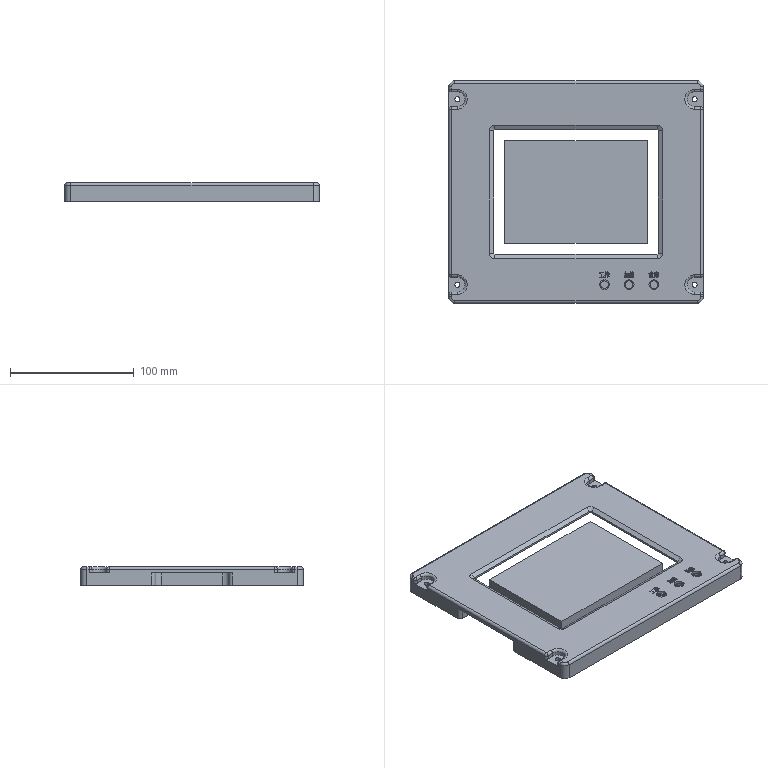NC program | Mastercam | posted with a generic post | part box 206 x 180 x 15 mm
Lines 737 to 1835 of 42274:
(4 BNOS |TOOL - 1|DIA. OFF. - 1|LEN. - 1|TOOL DIA. - 4.)
N1542 T1 M6
N1544 G0 G54 G90 X68.664 Y49.5 C0. B0. S10000 M3
N1546 G43 H1 Z24.953
N1548 Z4.953
N1550 G1 Z-.047 F600.
N1552 X68.643 Y49.851 F4000.
N1554 X68.576 Y50.211
N1556 X68.459 Y50.573
N1558 X68.339 Y50.838
N1560 X68.189 Y51.095
N1562 X68.012 Y51.337
N1564 X67.811 Y51.561
N1566 X67.587 Y51.762
N1568 X67.345 Y51.939
N1570 X67.088 Y52.089
N1572 X66.823 Y52.209
N1574 X66.461 Y52.326
N1576 X66.101 Y52.393
N1578 X65.75 Y52.414
N1580 X-65.75
N1582 X-66.101 Y52.393
N1584 X-66.461 Y52.326
N1586 X-66.823 Y52.209
N1588 X-67.088 Y52.089
N1590 X-67.345 Y51.939
N1592 X-67.587 Y51.762
N1594 X-67.811 Y51.561
N1596 X-68.012 Y51.337
N1598 X-68.189 Y51.095
N1600 X-68.339 Y50.838
N1602 X-68.459 Y50.573
N1604 X-68.576 Y50.211
N1606 X-68.643 Y49.851
N1608 X-68.664 Y49.5
N1610 Y-49.5
N1612 X-68.347
N1614 Z-.231
N1616 Y49.5
N1618 X-68.328 Y49.813
N1620 X-68.268 Y50.134
N1622 X-68.164 Y50.456
N1624 X-68.056 Y50.693
N1626 X-67.923 Y50.921
N1628 X-67.766 Y51.137
N1630 X-67.586 Y51.336
N1632 X-67.387 Y51.516
N1634 X-67.171 Y51.673
N1636 X-66.943 Y51.806
N1638 X-66.706 Y51.914
N1640 X-66.384 Y52.018
N1642 X-66.063 Y52.078
N1644 X-65.75 Y52.097
N1646 X65.75
N1648 X66.063 Y52.078
N1650 X66.384 Y52.018
N1652 X66.706 Y51.914
N1654 X66.943 Y51.806
N1656 X67.171 Y51.673
N1658 X67.387 Y51.516
N1660 X67.586 Y51.336
N1662 X67.766 Y51.137
N1664 X67.923 Y50.921
N1666 X68.056 Y50.693
N1668 X68.164 Y50.456
N1670 X68.268 Y50.134
N1672 X68.328 Y49.813
N1674 X68.347 Y49.5
N1676 Y-49.5
N1678 X68.328 Y-49.813
N1680 X68.268 Y-50.134
N1682 X68.164 Y-50.456
N1684 X68.056 Y-50.693
N1686 X67.923 Y-50.921
N1688 X67.766 Y-51.137
N1690 X67.586 Y-51.336
N1692 X67.387 Y-51.516
N1694 X67.171 Y-51.673
N1696 X66.943 Y-51.806
N1698 X66.706 Y-51.914
N1700 X66.384 Y-52.018
N1702 X66.063 Y-52.078
N1704 X65.75 Y-52.097
N1706 X-65.75
N1708 X-66.063 Y-52.078
N1710 X-66.384 Y-52.018
N1712 X-66.706 Y-51.914
N1714 X-66.943 Y-51.806
N1716 X-67.171 Y-51.673
N1718 X-67.387 Y-51.516
N1720 X-67.586 Y-51.336
N1722 X-67.766 Y-51.137
N1724 X-67.923 Y-50.921
N1726 X-68.056 Y-50.693
N1728 X-68.164 Y-50.456
N1730 X-68.268 Y-50.134
N1732 X-68.328 Y-49.813
N1734 X-68.347 Y-49.5
N1736 X-68.058
N1738 Z-.397
N1740 X-68.041 Y-49.778
N1742 X-67.988 Y-50.063
N1744 X-67.896 Y-50.35
N1746 X-67.8 Y-50.56
N1748 X-67.682 Y-50.763
N1750 X-67.542 Y-50.955
N1752 X-67.382 Y-51.132
N1754 X-67.205 Y-51.292
N1756 X-67.013 Y-51.432
N1758 X-66.81 Y-51.55
N1760 X-66.6 Y-51.646
N1762 X-66.313 Y-51.738
N1764 X-66.028 Y-51.791
N1766 X-65.75 Y-51.808
N1768 X65.75
N1770 X66.028 Y-51.791
N1772 X66.313 Y-51.738
N1774 X66.6 Y-51.646
N1776 X66.81 Y-51.55
N1778 X67.013 Y-51.432
N1780 X67.205 Y-51.292
N1782 X67.382 Y-51.132
N1784 X67.542 Y-50.955
N1786 X67.682 Y-50.763
N1788 X67.8 Y-50.56
N1790 X67.896 Y-50.35
N1792 X67.988 Y-50.063
N1794 X68.041 Y-49.778
N1796 X68.058 Y-49.5
N1798 Y49.5
N1800 X68.041 Y49.778
N1802 X67.988 Y50.063
N1804 X67.896 Y50.35
N1806 X67.8 Y50.56
N1808 X67.682 Y50.763
N1810 X67.542 Y50.955
N1812 X67.382 Y51.132
N1814 X67.205 Y51.292
N1816 X67.013 Y51.432
N1818 X66.81 Y51.55
N1820 X66.6 Y51.646
N1822 X66.313 Y51.738
N1824 X66.028 Y51.791
N1826 X65.75 Y51.808
N1828 X-65.75
N1830 X-66.028 Y51.791
N1832 X-66.313 Y51.738
N1834 X-66.6 Y51.646
N1836 X-66.81 Y51.55
N1838 X-67.013 Y51.432
N1840 X-67.205 Y51.292
N1842 X-67.382 Y51.132
N1844 X-67.542 Y50.955
N1846 X-67.682 Y50.763
N1848 X-67.8 Y50.56
N1850 X-67.896 Y50.35
N1852 X-67.988 Y50.063
N1854 X-68.041 Y49.778
N1856 X-68.058 Y49.5
N1858 Y-49.5
N1860 X-67.74
N1862 Z-.581
N1864 Y49.5
N1866 X-67.726 Y49.74
N1868 X-67.68 Y49.986
N1870 X-67.601 Y50.233
N1872 X-67.518 Y50.414
N1874 X-67.416 Y50.589
N1876 X-67.295 Y50.755
N1878 X-67.157 Y50.907
N1880 X-67.005 Y51.045
N1882 X-66.839 Y51.166
N1884 X-66.664 Y51.268
N1886 X-66.483 Y51.351
N1888 X-66.236 Y51.43
N1890 X-65.99 Y51.476
N1892 X-65.75 Y51.49
N1894 X65.75
N1896 X65.99 Y51.476
N1898 X66.236 Y51.43
N1900 X66.483 Y51.351
N1902 X66.664 Y51.268
N1904 X66.839 Y51.166
N1906 X67.005 Y51.045
N1908 X67.157 Y50.907
N1910 X67.295 Y50.755
N1912 X67.416 Y50.589
N1914 X67.518 Y50.414
N1916 X67.601 Y50.233
N1918 X67.68 Y49.986
N1920 X67.726 Y49.74
N1922 X67.74 Y49.5
N1924 Y-49.5
N1926 X67.726 Y-49.74
N1928 X67.68 Y-49.986
N1930 X67.601 Y-50.233
N1932 X67.518 Y-50.414
N1934 X67.416 Y-50.589
N1936 X67.295 Y-50.755
N1938 X67.157 Y-50.907
N1940 X67.005 Y-51.045
N1942 X66.839 Y-51.166
N1944 X66.664 Y-51.268
N1946 X66.483 Y-51.351
N1948 X66.236 Y-51.43
N1950 X65.99 Y-51.476
N1952 X65.75 Y-51.49
N1954 X-65.75
N1956 X-65.99 Y-51.476
N1958 X-66.236 Y-51.43
N1960 X-66.483 Y-51.351
N1962 X-66.664 Y-51.268
N1964 X-66.839 Y-51.166
N1966 X-67.005 Y-51.045
N1968 X-67.157 Y-50.907
N1970 X-67.295 Y-50.755
N1972 X-67.416 Y-50.589
N1974 X-67.518 Y-50.414
N1976 X-67.601 Y-50.233
N1978 X-67.68 Y-49.986
N1980 X-67.726 Y-49.74
N1982 X-67.74 Y-49.5
N1984 X-67.423
N1986 Z-.764
N1988 X-67.411 Y-49.701
N1990 X-67.372 Y-49.908
N1992 X-67.305 Y-50.116
N1994 X-67.236 Y-50.268
N1996 X-67.15 Y-50.415
N1998 X-67.049 Y-50.554
N2000 X-66.933 Y-50.683
N2002 X-66.804 Y-50.799
N2004 X-66.665 Y-50.9
N2006 X-66.518 Y-50.986
N2008 X-66.366 Y-51.055
N2010 X-66.158 Y-51.122
N2012 X-65.951 Y-51.161
N2014 X-65.75 Y-51.173
N2016 X65.75
N2018 X65.951 Y-51.161
N2020 X66.158 Y-51.122
N2022 X66.366 Y-51.055
N2024 X66.518 Y-50.986
N2026 X66.665 Y-50.9
N2028 X66.804 Y-50.799
N2030 X66.933 Y-50.683
N2032 X67.049 Y-50.554
N2034 X67.15 Y-50.415
N2036 X67.236 Y-50.268
N2038 X67.305 Y-50.116
N2040 X67.372 Y-49.908
N2042 X67.411 Y-49.701
N2044 X67.423 Y-49.5
N2046 Y49.5
N2048 X67.411 Y49.701
N2050 X67.372 Y49.908
N2052 X67.305 Y50.116
N2054 X67.236 Y50.268
N2056 X67.15 Y50.415
N2058 X67.049 Y50.554
N2060 X66.933 Y50.683
N2062 X66.804 Y50.799
N2064 X66.665 Y50.9
N2066 X66.518 Y50.986
N2068 X66.366 Y51.055
N2070 X66.158 Y51.122
N2072 X65.951 Y51.161
N2074 X65.75 Y51.173
N2076 X-65.75
N2078 X-65.951 Y51.161
N2080 X-66.158 Y51.122
N2082 X-66.366 Y51.055
N2084 X-66.518 Y50.986
N2086 X-66.665 Y50.9
N2088 X-66.804 Y50.799
N2090 X-66.933 Y50.683
N2092 X-67.049 Y50.554
N2094 X-67.15 Y50.415
N2096 X-67.236 Y50.268
N2098 X-67.305 Y50.116
N2100 X-67.372 Y49.908
N2102 X-67.411 Y49.701
N2104 X-67.423 Y49.5
N2106 Y-49.5
N2108 X-67.105
N2110 Z-.947
N2112 Y49.5
N2114 X-67.095 Y49.663
N2116 X-67.064 Y49.831
N2118 X-67.01 Y49.999
N2120 X-66.954 Y50.122
N2122 X-66.884 Y50.242
N2124 X-66.802 Y50.354
N2126 X-66.708 Y50.458
N2128 X-66.604 Y50.552
N2130 X-66.492 Y50.634
N2132 X-66.372 Y50.704
N2134 X-66.249 Y50.76
N2136 X-66.081 Y50.814
N2138 X-65.913 Y50.845
N2140 X-65.75 Y50.855
N2142 X65.75
N2144 X65.913 Y50.845
N2146 X66.081 Y50.814
N2148 X66.249 Y50.76
N2150 X66.372 Y50.704
N2152 X66.492 Y50.634
N2154 X66.604 Y50.552
N2156 X66.708 Y50.458
N2158 X66.802 Y50.354
N2160 X66.884 Y50.242
N2162 X66.954 Y50.122
N2164 X67.01 Y49.999
N2166 X67.064 Y49.831
N2168 X67.095 Y49.663
N2170 X67.105 Y49.5
N2172 Y-49.5
N2174 X67.095 Y-49.663
N2176 X67.064 Y-49.831
N2178 X67.01 Y-49.999
N2180 X66.954 Y-50.122
N2182 X66.884 Y-50.242
N2184 X66.802 Y-50.354
N2186 X66.708 Y-50.458
N2188 X66.604 Y-50.552
N2190 X66.492 Y-50.634
N2192 X66.372 Y-50.704
N2194 X66.249 Y-50.76
N2196 X66.081 Y-50.814
N2198 X65.913 Y-50.845
N2200 X65.75 Y-50.855
N2202 X-65.75
N2204 X-65.913 Y-50.845
N2206 X-66.081 Y-50.814
N2208 X-66.249 Y-50.76
N2210 X-66.372 Y-50.704
N2212 X-66.492 Y-50.634
N2214 X-66.604 Y-50.552
N2216 X-66.708 Y-50.458
N2218 X-66.802 Y-50.354
N2220 X-66.884 Y-50.242
N2222 X-66.954 Y-50.122
N2224 X-67.01 Y-49.999
N2226 X-67.064 Y-49.831
N2228 X-67.095 Y-49.663
N2230 X-67.105 Y-49.5
N2232 X-66.788
N2234 Z-1.131
N2236 X-66.78 Y-49.625
N2238 X-66.756 Y-49.753
N2240 X-66.715 Y-49.882
N2242 X-66.672 Y-49.977
N2244 X-66.619 Y-50.068
N2246 X-66.556 Y-50.154
N2248 X-66.484 Y-50.234
N2250 X-66.404 Y-50.306
N2252 X-66.318 Y-50.369
N2254 X-66.227 Y-50.422
N2256 X-66.132 Y-50.465
N2258 X-66.003 Y-50.506
N2260 X-65.875 Y-50.53
N2262 X-65.75 Y-50.538
N2264 X65.75
N2266 X65.875 Y-50.53
N2268 X66.003 Y-50.506
N2270 X66.132 Y-50.465
N2272 X66.227 Y-50.422
N2274 X66.318 Y-50.369
N2276 X66.404 Y-50.306
N2278 X66.484 Y-50.234
N2280 X66.556 Y-50.154
N2282 X66.619 Y-50.068
N2284 X66.672 Y-49.977
N2286 X66.715 Y-49.882
N2288 X66.756 Y-49.753
N2290 X66.78 Y-49.625
N2292 X66.788 Y-49.5
N2294 Y49.5
N2296 X66.78 Y49.625
N2298 X66.756 Y49.753
N2300 X66.715 Y49.882
N2302 X66.672 Y49.977
N2304 X66.619 Y50.068
N2306 X66.556 Y50.154
N2308 X66.484 Y50.234
N2310 X66.404 Y50.306
N2312 X66.318 Y50.369
N2314 X66.227 Y50.422
N2316 X66.132 Y50.465
N2318 X66.003 Y50.506
N2320 X65.875 Y50.53
N2322 X65.75 Y50.538
N2324 X-65.75
N2326 X-65.875 Y50.53
N2328 X-66.003 Y50.506
N2330 X-66.132 Y50.465
N2332 X-66.227 Y50.422
N2334 X-66.318 Y50.369
N2336 X-66.404 Y50.306
N2338 X-66.484 Y50.234
N2340 X-66.556 Y50.154
N2342 X-66.619 Y50.068
N2344 X-66.672 Y49.977
N2346 X-66.715 Y49.882
N2348 X-66.756 Y49.753
N2350 X-66.78 Y49.625
N2352 X-66.788 Y49.5
N2354 Y-49.5
N2356 X-66.47
N2358 Z-1.314
N2360 Y49.5
N2362 X-66.465 Y49.587
N2364 X-66.448 Y49.676
N2366 X-66.42 Y49.765
N2368 X-66.39 Y49.831
N2370 X-66.353 Y49.894
N2372 X-66.309 Y49.954
N2374 X-66.259 Y50.009
N2376 X-66.204 Y50.059
N2378 X-66.144 Y50.103
N2380 X-66.081 Y50.14
N2382 X-66.015 Y50.17
N2384 X-65.926 Y50.198
N2386 X-65.837 Y50.215
N2388 X-65.75 Y50.22
N2390 X65.75
N2392 X65.837 Y50.215
N2394 X65.926 Y50.198
N2396 X66.015 Y50.17
N2398 X66.081 Y50.14
N2400 X66.144 Y50.103
N2402 X66.204 Y50.059
N2404 X66.259 Y50.009
N2406 X66.309 Y49.954
N2408 X66.353 Y49.894
N2410 X66.39 Y49.831
N2412 X66.42 Y49.765
N2414 X66.448 Y49.676
N2416 X66.465 Y49.587
N2418 X66.47 Y49.5
N2420 Y-49.5
N2422 X66.465 Y-49.587
N2424 X66.448 Y-49.676
N2426 X66.42 Y-49.765
N2428 X66.39 Y-49.831
N2430 X66.353 Y-49.894
N2432 X66.309 Y-49.954
N2434 X66.259 Y-50.009
N2436 X66.204 Y-50.059
N2438 X66.144 Y-50.103
N2440 X66.081 Y-50.14
N2442 X66.015 Y-50.17
N2444 X65.926 Y-50.198
N2446 X65.837 Y-50.215
N2448 X65.75 Y-50.22
N2450 X-65.75
N2452 X-65.837 Y-50.215
N2454 X-65.926 Y-50.198
N2456 X-66.015 Y-50.17
N2458 X-66.081 Y-50.14
N2460 X-66.144 Y-50.103
N2462 X-66.204 Y-50.059
N2464 X-66.259 Y-50.009
N2466 X-66.309 Y-49.954
N2468 X-66.353 Y-49.894
N2470 X-66.39 Y-49.831
N2472 X-66.42 Y-49.765
N2474 X-66.448 Y-49.676
N2476 X-66.465 Y-49.587
N2478 X-66.47 Y-49.5
N2480 X-66.153
N2482 Z-1.497
N2484 X-66.15 Y-49.548
N2486 X-66.14 Y-49.598
N2488 X-66.124 Y-49.648
N2490 X-66.108 Y-49.685
N2492 X-66.087 Y-49.72
N2494 X-66.063 Y-49.754
N2496 X-66.035 Y-49.785
N2498 X-66.004 Y-49.813
N2500 X-65.97 Y-49.837
N2502 X-65.935 Y-49.858
N2504 X-65.898 Y-49.874
N2506 X-65.848 Y-49.89
N2508 X-65.798 Y-49.9
N2510 X-65.75 Y-49.903
N2512 X65.75
N2514 X65.798 Y-49.9
N2516 X65.848 Y-49.89
N2518 X65.898 Y-49.874
N2520 X65.935 Y-49.858
N2522 X65.97 Y-49.837
N2524 X66.004 Y-49.813
N2526 X66.035 Y-49.785
N2528 X66.063 Y-49.754
N2530 X66.087 Y-49.72
N2532 X66.108 Y-49.685
N2534 X66.124 Y-49.648
N2536 X66.14 Y-49.598
N2538 X66.15 Y-49.548
N2540 X66.153 Y-49.5
N2542 Y49.5
N2544 X66.15 Y49.548
N2546 X66.14 Y49.598
N2548 X66.124 Y49.648
N2550 X66.108 Y49.685
N2552 X66.087 Y49.72
N2554 X66.063 Y49.754
N2556 X66.035 Y49.785
N2558 X66.004 Y49.813
N2560 X65.97 Y49.837
N2562 X65.935 Y49.858
N2564 X65.898 Y49.874
N2566 X65.848 Y49.89
N2568 X65.798 Y49.9
N2570 X65.75 Y49.903
N2572 X-65.75
N2574 X-65.798 Y49.9
N2576 X-65.848 Y49.89
N2578 X-65.898 Y49.874
N2580 X-65.935 Y49.858
N2582 X-65.97 Y49.837
N2584 X-66.004 Y49.813
N2586 X-66.035 Y49.785
N2588 X-66.063 Y49.754
N2590 X-66.087 Y49.72
N2592 X-66.108 Y49.685
N2594 X-66.124 Y49.648
N2596 X-66.14 Y49.598
N2598 X-66.15 Y49.548
N2600 X-66.153 Y49.5
N2602 Y-49.5
N2604 X-65.835
N2606 Z-1.681
N2608 Y49.5
N2610 X-65.834 Y49.51
N2612 X-65.833 Y49.521
N2614 X-65.829 Y49.531
N2616 X-65.826 Y49.539
N2618 X-65.821 Y49.547
N2620 X-65.816 Y49.554
N2622 X-65.81 Y49.56
N2624 X-65.804 Y49.566
N2626 X-65.797 Y49.571
N2628 X-65.789 Y49.576
N2630 X-65.781 Y49.579
N2632 X-65.771 Y49.583
N2634 X-65.76 Y49.584
N2636 X-65.75 Y49.585
N2638 X65.75
N2640 X65.76 Y49.584
N2642 X65.771 Y49.583
N2644 X65.781 Y49.579
N2646 X65.789 Y49.576
N2648 X65.797 Y49.571
N2650 X65.804 Y49.566
N2652 X65.81 Y49.56
N2654 X65.816 Y49.554
N2656 X65.821 Y49.547
N2658 X65.826 Y49.539
N2660 X65.829 Y49.531
N2662 X65.833 Y49.521
N2664 X65.834 Y49.51
N2666 X65.835 Y49.5
N2668 Y-49.5
N2670 X65.834 Y-49.51
N2672 X65.833 Y-49.521
N2674 X65.829 Y-49.531
N2676 X65.826 Y-49.539
N2678 X65.821 Y-49.547
N2680 X65.816 Y-49.554
N2682 X65.81 Y-49.56
N2684 X65.804 Y-49.566
N2686 X65.797 Y-49.571
N2688 X65.789 Y-49.576
N2690 X65.781 Y-49.579
N2692 X65.771 Y-49.583
N2694 X65.76 Y-49.584
N2696 X65.75 Y-49.585
N2698 X-65.75
N2700 X-65.76 Y-49.584
N2702 X-65.771 Y-49.583
N2704 X-65.781 Y-49.579
N2706 X-65.789 Y-49.576
N2708 X-65.797 Y-49.571
N2710 X-65.804 Y-49.566
N2712 X-65.81 Y-49.56
N2714 X-65.816 Y-49.554
N2716 X-65.821 Y-49.547
N2718 X-65.826 Y-49.539
N2720 X-65.829 Y-49.531
N2722 X-65.833 Y-49.521
N2724 X-65.834 Y-49.51
N2726 X-65.835 Y-49.5
N2728 X-65.558 Y-49.268
N2730 Z-1.864
N2732 X65.518
N2734 Y49.268
N2736 X-65.518
N2738 Y-49.308
N2740 Z-1.846
N2742 X-65.2 Y-48.99
N2744 Z-2.047
N2746 Y48.95
N2748 X65.2
N2750 Y-48.95
N2752 X-65.24
N2754 G0 Z2.953
N2756 Z22.953
N2758 Z24.953
N2760 X-65.75 Y-52.414
N2762 Z4.953
N2764 G1 Z-.047 F600.
N2766 X-66.101 Y-52.393 F4000.
N2768 X-66.461 Y-52.326
N2770 X-66.823 Y-52.209
N2772 X-67.088 Y-52.089
N2774 X-67.345 Y-51.939
N2776 X-67.587 Y-51.762
N2778 X-67.811 Y-51.561
N2780 X-68.012 Y-51.337
N2782 X-68.189 Y-51.095
N2784 X-68.339 Y-50.838
N2786 X-68.459 Y-50.573
N2788 X-68.576 Y-50.211
N2790 X-68.643 Y-49.851
N2792 X-68.664 Y-49.5
N2794 G0 Z4.953
N2796 Z24.953
N2798 X-65.75 Y-52.414
N2800 Z4.953
N2802 G1 Z-.047 F600.
N2804 X65.75 F4000.
N2806 X66.101 Y-52.393
N2808 X66.461 Y-52.326
N2810 X66.823 Y-52.209
N2812 X67.088 Y-52.089
N2814 X67.345 Y-51.939
N2816 X67.587 Y-51.762
N2818 X67.811 Y-51.561
N2820 X68.012 Y-51.337
N2822 X68.189 Y-51.095
N2824 X68.339 Y-50.838
N2826 X68.459 Y-50.573
N2828 X68.576 Y-50.211
N2830 X68.643 Y-49.851
N2832 X68.664 Y-49.5
N2834 Y49.5
N2836 G0 Z4.953
N2838 Z24.953
N2840 Z37.5
N2842 X0. Y-89.045
N2844 Z20.
N2846 Z10.
N2848 G1 Z0. F600.
N2850 X-98. F4000.
N2852 X-98.363 Y-89.029
N2854 X-98.736 Y-88.977
N2856 X-99.113 Y-88.889
N2858 X-99.489 Y-88.761
N2860 X-99.858 Y-88.593
N2862 X-100.213 Y-88.386
N2864 X-100.55 Y-88.14
N2866 X-100.86 Y-87.86
N2868 X-101.14 Y-87.55
N2870 X-101.386 Y-87.213
N2872 X-101.593 Y-86.858
N2874 X-101.761 Y-86.489
N2876 X-101.889 Y-86.113
N2878 X-101.977 Y-85.736
N2880 X-102.029 Y-85.363
N2882 X-102.045 Y-85.
N2884 Y-83.
N2886 X-101.739 Y-82.261
N2888 X-101. Y-81.955
N2890 X-96.
N2892 X-95.6 Y-81.943
N2894 X-95.178 Y-81.906
N2896 X-94.687 Y-81.829
N2898 X-94.281 Y-81.739
N2900 X-93.879 Y-81.624
N2902 X-93.485 Y-81.484
N2904 X-93.098 Y-81.32
N2906 X-92.721 Y-81.133
N2908 X-92.355 Y-80.923
N2910 X-92.002 Y-80.691
N2912 X-91.706 Y-80.471
N2914 X-91.346 Y-80.168
N2916 X-90.998 Y-79.832
N2918 X-90.746 Y-79.556
N2920 X-90.476 Y-79.225
N2922 X-90.226 Y-78.876
N2924 X-89.998 Y-78.513
N2926 X-89.792 Y-78.135
N2928 X-89.61 Y-77.745
N2930 X-89.452 Y-77.343
N2932 X-89.319 Y-76.932
N2934 X-89.211 Y-76.511
N2936 X-89.13 Y-76.085
N2938 X-89.076 Y-75.653
N2940 X-89.049 Y-75.218
N2942 X-89.051 Y-74.721
N2944 X-89.08 Y-74.304
N2946 X-89.134 Y-73.891
N2948 X-89.218 Y-73.458
N2950 X-89.329 Y-73.034
N2952 X-89.468 Y-72.612
N2954 X-89.632 Y-72.205
N2956 X-89.824 Y-71.802
N2958 X-90.039 Y-71.418
N2960 X-90.283 Y-71.04
N2962 X-90.546 Y-70.686
N2964 X-90.838 Y-70.34
N2966 X-91.144 Y-70.021
N2968 X-91.481 Y-69.713
N2970 X-91.827 Y-69.436
N2972 X-92.196 Y-69.178
N2974 X-92.567 Y-68.952
N2976 X-92.938 Y-68.756
N2978 X-93.306 Y-68.588
N2980 X-93.743 Y-68.422
N2982 X-94.17 Y-68.29
N2984 X-94.631 Y-68.182
N2986 X-95.073 Y-68.108
N2988 X-95.55 Y-68.06
N2990 X-96. Y-68.045
N2992 X-101.
N2994 X-101.739 Y-67.739
N2996 X-102.045 Y-67.
N2998 Y67.
N3000 X-101.739 Y67.739
N3002 X-101. Y68.045
N3004 X-96.
N3006 X-95.6 Y68.057
N3008 X-95.178 Y68.094
N3010 X-94.687 Y68.171
N3012 X-94.281 Y68.261
N3014 X-93.879 Y68.376
N3016 X-93.485 Y68.516
N3018 X-93.098 Y68.68
N3020 X-92.721 Y68.867
N3022 X-92.355 Y69.077
N3024 X-92.002 Y69.309
N3026 X-91.706 Y69.529
N3028 X-91.346 Y69.832
N3030 X-90.998 Y70.168
N3032 X-90.746 Y70.444
N3034 X-90.476 Y70.775
N3036 X-90.226 Y71.124
N3038 X-89.998 Y71.487
N3040 X-89.792 Y71.865
N3042 X-89.61 Y72.255
N3044 X-89.452 Y72.657
N3046 X-89.319 Y73.068
N3048 X-89.211 Y73.489
N3050 X-89.13 Y73.915
N3052 X-89.076 Y74.347
N3054 X-89.049 Y74.782
N3056 X-89.051 Y75.279
N3058 X-89.08 Y75.696
N3060 X-89.134 Y76.109
N3062 X-89.218 Y76.542
N3064 X-89.329 Y76.966
N3066 X-89.468 Y77.388
N3068 X-89.632 Y77.795
N3070 X-89.824 Y78.198
N3072 X-90.039 Y78.582
N3074 X-90.283 Y78.96
N3076 X-90.546 Y79.314
N3078 X-90.838 Y79.66
N3080 X-91.144 Y79.979
N3082 X-91.481 Y80.287
N3084 X-91.827 Y80.564
N3086 X-92.196 Y80.822
N3088 X-92.567 Y81.048
N3090 X-92.938 Y81.244
N3092 X-93.306 Y81.412
N3094 X-93.743 Y81.578
N3096 X-94.17 Y81.71
N3098 X-94.631 Y81.818
N3100 X-95.073 Y81.892
N3102 X-95.55 Y81.94
N3104 X-96. Y81.955
N3106 X-101.
N3108 X-101.739 Y82.261
N3110 X-102.045 Y83.
N3112 Y85.
N3114 X-102.029 Y85.363
N3116 X-101.977 Y85.736
N3118 X-101.889 Y86.113
N3120 X-101.761 Y86.489
N3122 X-101.593 Y86.858
N3124 X-101.386 Y87.213
N3126 X-101.14 Y87.55
N3128 X-100.86 Y87.86
N3130 X-100.55 Y88.14
N3132 X-100.213 Y88.386
N3134 X-99.858 Y88.593
N3136 X-99.489 Y88.761
N3138 X-99.113 Y88.889
N3140 X-98.736 Y88.977
N3142 X-98.363 Y89.029
N3144 X-98. Y89.045
N3146 X98.
N3148 X98.363 Y89.029
N3150 X98.736 Y88.977
N3152 X99.113 Y88.889
N3154 X99.489 Y88.761
N3156 X99.858 Y88.593
N3158 X100.213 Y88.386
N3160 X100.55 Y88.14
N3162 X100.86 Y87.86
N3164 X101.14 Y87.55
N3166 X101.386 Y87.213
N3168 X101.593 Y86.858
N3170 X101.761 Y86.489
N3172 X101.889 Y86.113
N3174 X101.977 Y85.736
N3176 X102.029 Y85.363
N3178 X102.045 Y85.
N3180 Y83.
N3182 X101.739 Y82.261
N3184 X101. Y81.955
N3186 X96.
N3188 X95.6 Y81.943
N3190 X95.178 Y81.906
N3192 X94.687 Y81.829
N3194 X94.281 Y81.739
N3196 X93.879 Y81.624
N3198 X93.485 Y81.484
N3200 X93.098 Y81.32
N3202 X92.721 Y81.133
N3204 X92.355 Y80.923
N3206 X92.002 Y80.691
N3208 X91.706 Y80.471
N3210 X91.346 Y80.168
N3212 X90.998 Y79.832
N3214 X90.746 Y79.556
N3216 X90.476 Y79.225
N3218 X90.226 Y78.876
N3220 X89.998 Y78.513
N3222 X89.792 Y78.135
N3224 X89.61 Y77.745
N3226 X89.452 Y77.343
N3228 X89.319 Y76.932
N3230 X89.211 Y76.511
N3232 X89.13 Y76.085
N3234 X89.076 Y75.653
N3236 X89.049 Y75.218
N3238 X89.051 Y74.721
N3240 X89.08 Y74.304
N3242 X89.134 Y73.891
N3244 X89.218 Y73.458
N3246 X89.329 Y73.034
N3248 X89.468 Y72.612
N3250 X89.632 Y72.205
N3252 X89.824 Y71.802
N3254 X90.039 Y71.418
N3256 X90.283 Y71.04
N3258 X90.546 Y70.686
N3260 X90.838 Y70.34
N3262 X91.144 Y70.021
N3264 X91.481 Y69.713
N3266 X91.827 Y69.436
N3268 X92.196 Y69.178
N3270 X92.567 Y68.952
N3272 X92.938 Y68.756
N3274 X93.306 Y68.588
N3276 X93.743 Y68.422
N3278 X94.17 Y68.29
N3280 X94.631 Y68.182
N3282 X95.073 Y68.108
N3284 X95.55 Y68.06
N3286 X96. Y68.045
N3288 X101.
N3290 X101.739 Y67.739
N3292 X102.045 Y67.
N3294 Y-67.
N3296 X101.739 Y-67.739
N3298 X101. Y-68.045
N3300 X96.
N3302 X95.6 Y-68.057
N3304 X95.178 Y-68.094
N3306 X94.687 Y-68.171
N3308 X94.281 Y-68.261
N3310 X93.879 Y-68.376
N3312 X93.485 Y-68.516
N3314 X93.098 Y-68.68
N3316 X92.721 Y-68.867
N3318 X92.355 Y-69.077
N3320 X92.002 Y-69.309
N3322 X91.706 Y-69.529
N3324 X91.346 Y-69.832
N3326 X90.998 Y-70.168
N3328 X90.746 Y-70.444
N3330 X90.476 Y-70.775
N3332 X90.226 Y-71.124
N3334 X89.998 Y-71.487
N3336 X89.792 Y-71.865
N3338 X89.61 Y-72.255
N3340 X89.452 Y-72.657
N3342 X89.319 Y-73.068
N3344 X89.211 Y-73.489
N3346 X89.13 Y-73.915
N3348 X89.076 Y-74.347
N3350 X89.049 Y-74.782
N3352 X89.051 Y-75.279
N3354 X89.08 Y-75.696
N3356 X89.134 Y-76.109
N3358 X89.218 Y-76.542
N3360 X89.329 Y-76.966
N3362 X89.468 Y-77.388
N3364 X89.632 Y-77.795
N3366 X89.824 Y-78.198
N3368 X90.039 Y-78.582
N3370 X90.283 Y-78.96
N3372 X90.546 Y-79.314
N3374 X90.838 Y-79.66
N3376 X91.144 Y-79.979
N3378 X91.481 Y-80.287
N3380 X91.827 Y-80.564
N3382 X92.196 Y-80.822
N3384 X92.567 Y-81.048
N3386 X92.938 Y-81.244
N3388 X93.306 Y-81.412
N3390 X93.743 Y-81.578
N3392 X94.17 Y-81.71
N3394 X94.631 Y-81.818
N3396 X95.073 Y-81.892
N3398 X95.55 Y-81.94
N3400 X96. Y-81.955
N3402 X101.
N3404 X101.739 Y-82.261
N3406 X102.045 Y-83.
N3408 Y-85.
N3410 X102.029 Y-85.363
N3412 X101.977 Y-85.736
N3414 X101.889 Y-86.113
N3416 X101.761 Y-86.489
N3418 X101.593 Y-86.858
N3420 X101.386 Y-87.213
N3422 X101.14 Y-87.55
N3424 X100.86 Y-87.86
N3426 X100.55 Y-88.14
N3428 X100.213 Y-88.386
N3430 X99.858 Y-88.593
N3432 X99.489 Y-88.761
N3434 X99.113 Y-88.889
N3436 X98.736 Y-88.977
N3438 X98.363 Y-89.029
N3440 X98. Y-89.045
N3442 X0.
N3444 X-.033 Y-89.05 Z-.001
N3446 X-.046 Y-89.056
N3448 X-.057 Y-89.064
N3450 X-.065 Y-89.075 Z-.002
N3452 X-.071 Y-89.087
N3454 X-.075 Y-89.12 Z-.003
N3456 X-.071 Y-89.153 Z-.005
N3458 X-.065 Y-89.166
N3460 X-.057 Y-89.177 Z-.006
N3462 X-.046 Y-89.185
N3464 X-.033 Y-89.191
N3466 X0. Y-89.196
N3468 X98.
N3470 X98.377 Y-89.179
N3472 X98.763 Y-89.125
N3474 X99.154 Y-89.034
N3476 X99.544 Y-88.901
N3478 X99.927 Y-88.727
N3480 X100.296 Y-88.512
N3482 X100.644 Y-88.257
N3484 X100.967 Y-87.967
N3486 X101.257 Y-87.644
N3488 X101.512 Y-87.296
N3490 X101.727 Y-86.927
N3492 X101.901 Y-86.544
N3494 X102.034 Y-86.154
N3496 X102.125 Y-85.763
N3498 X102.179 Y-85.377
N3500 X102.196 Y-85.
N3502 Y-83.
N3504 X102.106 Y-82.544
N3506 X101.995 Y-82.337
N3508 X101.845 Y-82.154
N3510 X101.662 Y-82.005
N3512 X101.455 Y-81.894
N3514 X101. Y-81.804
N3516 X96.
N3518 X95.554 Y-81.789
N3520 X95.081 Y-81.742
N3522 X94.643 Y-81.667
N3524 X94.186 Y-81.558
N3526 X93.764 Y-81.426
N3528 X93.331 Y-81.259
N3530 X92.979 Y-81.096
N3532 X92.624 Y-80.907
N3534 X92.27 Y-80.69
N3536 X91.918 Y-80.443
N3538 X91.575 Y-80.169
N3540 X91.241 Y-79.863
N3542 X90.938 Y-79.547
N3544 X90.65 Y-79.203
N3546 X90.391 Y-78.851
N3548 X90.15 Y-78.476
N3550 X89.94 Y-78.094
N3552 X89.752 Y-77.693
N3554 X89.593 Y-77.288
N3556 X89.458 Y-76.87
N3558 X89.352 Y-76.449
N3560 X89.272 Y-76.019
N3562 X89.226 Y-75.639
N3564 X89.201 Y-75.256
N3566 X89.2 Y-74.784
N3568 X89.227 Y-74.353
N3570 X89.281 Y-73.925
N3572 X89.363 Y-73.503
N3574 X89.471 Y-73.087
N3576 X89.604 Y-72.68
N3578 X89.762 Y-72.283
N3580 X89.945 Y-71.897
N3582 X90.151 Y-71.524
N3584 X90.379 Y-71.166
N3586 X90.629 Y-70.823
N3588 X90.899 Y-70.497
N3590 X91.145 Y-70.233
N3592 X91.47 Y-69.923
N3594 X91.804 Y-69.643
N3596 X92.091 Y-69.431
N3598 X92.441 Y-69.201
N3600 X92.804 Y-68.994
N3602 X93.177 Y-68.809
N3604 X93.561 Y-68.648
N3606 X93.952 Y-68.511
N3608 X94.35 Y-68.399
N3610 X94.753 Y-68.311
N3612 X95.224 Y-68.24
N3614 X95.622 Y-68.206
N3616 X96. Y-68.196
N3618 X101.
N3620 X101.455 Y-68.106
N3622 X101.662 Y-67.995
N3624 X101.845 Y-67.846
N3626 X101.995 Y-67.663
N3628 X102.106 Y-67.456
N3630 X102.196 Y-67.
N3632 Y67.
N3634 X102.106 Y67.456
N3636 X101.995 Y67.663
N3638 X101.845 Y67.846
N3640 X101.662 Y67.995
N3642 X101.455 Y68.106
N3644 X101. Y68.196
N3646 X96.
N3648 X95.554 Y68.211
N3650 X95.081 Y68.258
N3652 X94.643 Y68.333
N3654 X94.186 Y68.442
N3656 X93.764 Y68.574
N3658 X93.331 Y68.741
N3660 X92.979 Y68.904
N3662 X92.624 Y69.093
N3664 X92.27 Y69.31
N3666 X91.918 Y69.557
N3668 X91.575 Y69.831
N3670 X91.241 Y70.137
N3672 X90.938 Y70.453
N3674 X90.65 Y70.797
N3676 X90.391 Y71.149
N3678 X90.15 Y71.524
N3680 X89.94 Y71.906
N3682 X89.752 Y72.307
N3684 X89.593 Y72.712
N3686 X89.458 Y73.13
N3688 X89.352 Y73.551
N3690 X89.272 Y73.981
N3692 X89.226 Y74.361
N3694 X89.201 Y74.744
N3696 X89.2 Y75.216
N3698 X89.227 Y75.647
N3700 X89.281 Y76.075
N3702 X89.363 Y76.497
N3704 X89.471 Y76.913
N3706 X89.604 Y77.32
N3708 X89.762 Y77.717
N3710 X89.945 Y78.103
N3712 X90.151 Y78.476
N3714 X90.379 Y78.834
N3716 X90.629 Y79.177
N3718 X90.899 Y79.503
N3720 X91.145 Y79.767
N3722 X91.47 Y80.077
N3724 X91.804 Y80.357
N3726 X92.091 Y80.569
N3728 X92.441 Y80.799
N3730 X92.804 Y81.006
N3732 X93.177 Y81.191
N3734 X93.561 Y81.352
N3736 X93.952 Y81.489